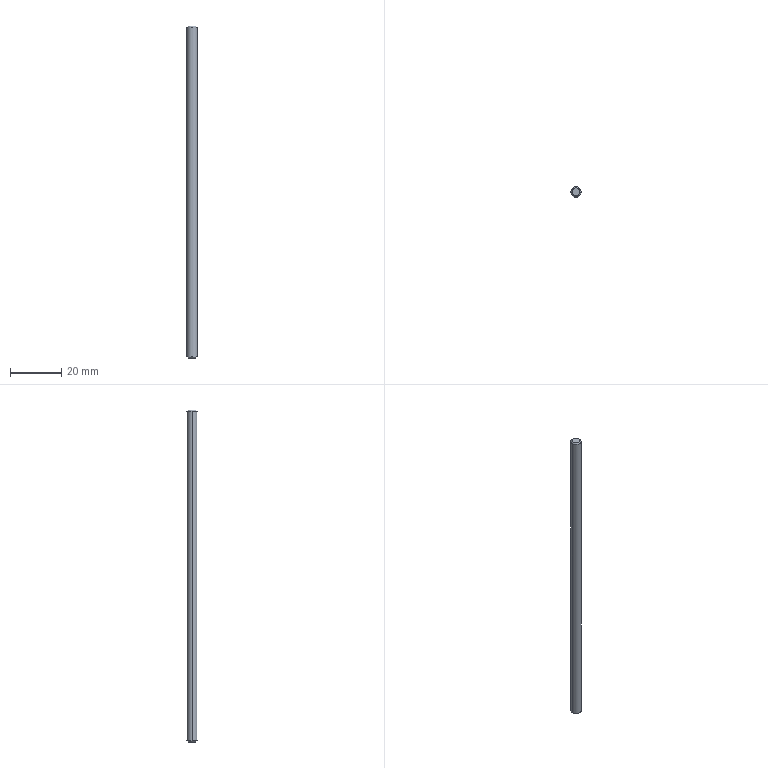Part | STEP file | 11-FG-B08311 | 1 solid | 8 faces | box 4 x 4 x 130 mm | volume 1631 mm3 | cone 4 | cylinder 2 | plane 2 | commonest cylinder face diameters 4 x2
STEP:
#1=CARTESIAN_POINT('',(-1.5,0.,0.));
#2=VERTEX_POINT('',#1);
#3=CARTESIAN_POINT('',(1.5,0.,0.));
#4=VERTEX_POINT('',#3);
#5=CARTESIAN_POINT('',(0.,0.,0.));
#6=DIRECTION('',(0.,0.,-1.));
#7=DIRECTION('',(1.,0.,0.));
#8=AXIS2_PLACEMENT_3D('',#5,#6,#7);
#9=CIRCLE('',#8,1.5);
#10=EDGE_CURVE('',#2,#4,#9,.T.);
#11=ORIENTED_EDGE('',*,*,#10,.F.);
#12=CARTESIAN_POINT('',(-2.,0.,0.5));
#13=VERTEX_POINT('',#12);
#14=CARTESIAN_POINT('',(-2.,0.,0.5));
#15=DIRECTION('',(-0.7071,0.,0.7071));
#16=VECTOR('',#15,1000.);
#17=LINE('',#14,#16);
#18=EDGE_CURVE('',#2,#13,#17,.T.);
#19=ORIENTED_EDGE('',*,*,#18,.T.);
#20=CARTESIAN_POINT('',(2.,0.,0.5));
#21=VERTEX_POINT('',#20);
#22=CARTESIAN_POINT('',(0.,0.,0.5));
#23=DIRECTION('',(0.,0.,1.));
#24=DIRECTION('',(1.,0.,0.));
#25=AXIS2_PLACEMENT_3D('',#22,#23,#24);
#26=CIRCLE('',#25,2.);
#27=EDGE_CURVE('',#21,#13,#26,.T.);
#28=ORIENTED_EDGE('',*,*,#27,.F.);
#29=CARTESIAN_POINT('',(2.,0.,0.5));
#30=DIRECTION('',(0.7071,0.,0.7071));
#31=VECTOR('',#30,1000.);
#32=LINE('',#29,#31);
#33=EDGE_CURVE('',#4,#21,#32,.T.);
#34=ORIENTED_EDGE('',*,*,#33,.F.);
#35=EDGE_LOOP('',(#11,#19,#28,#34));
#36=FACE_OUTER_BOUND('',#35,.T.);
#37=CARTESIAN_POINT('',(0.,0.,0.5));
#38=DIRECTION('',(0.,0.,1.));
#39=DIRECTION('',(1.,0.,0.));
#40=AXIS2_PLACEMENT_3D('',#37,#38,#39);
#41=CONICAL_SURFACE('',#40,2.,0.7854);
#42=ADVANCED_FACE('',(#36),#41,.T.);
#43=CARTESIAN_POINT('',(1.5,0.,130.));
#44=VERTEX_POINT('',#43);
#45=CARTESIAN_POINT('',(-1.5,0.,130.));
#46=VERTEX_POINT('',#45);
#47=CARTESIAN_POINT('',(0.,0.,130.));
#48=DIRECTION('',(0.,0.,1.));
#49=DIRECTION('',(1.,0.,0.));
#50=AXIS2_PLACEMENT_3D('',#47,#48,#49);
#51=CIRCLE('',#50,1.5);
#52=EDGE_CURVE('',#44,#46,#51,.T.);
#53=ORIENTED_EDGE('',*,*,#52,.F.);
#54=CARTESIAN_POINT('',(2.,0.,129.5));
#55=VERTEX_POINT('',#54);
#56=CARTESIAN_POINT('',(1.5,0.,130.));
#57=DIRECTION('',(0.7071,0.,-0.7071));
#58=VECTOR('',#57,1000.);
#59=LINE('',#56,#58);
#60=EDGE_CURVE('',#44,#55,#59,.T.);
#61=ORIENTED_EDGE('',*,*,#60,.T.);
#62=CARTESIAN_POINT('',(-2.,0.,129.5));
#63=VERTEX_POINT('',#62);
#64=CARTESIAN_POINT('',(0.,0.,129.5));
#65=DIRECTION('',(0.,0.,-1.));
#66=DIRECTION('',(1.,0.,0.));
#67=AXIS2_PLACEMENT_3D('',#64,#65,#66);
#68=CIRCLE('',#67,2.);
#69=EDGE_CURVE('',#63,#55,#68,.T.);
#70=ORIENTED_EDGE('',*,*,#69,.F.);
#71=CARTESIAN_POINT('',(-1.5,0.,130.));
#72=DIRECTION('',(-0.7071,0.,-0.7071));
#73=VECTOR('',#72,1000.);
#74=LINE('',#71,#73);
#75=EDGE_CURVE('',#46,#63,#74,.T.);
#76=ORIENTED_EDGE('',*,*,#75,.F.);
#77=EDGE_LOOP('',(#53,#61,#70,#76));
#78=FACE_OUTER_BOUND('',#77,.T.);
#79=CARTESIAN_POINT('',(0.,0.,130.));
#80=DIRECTION('',(0.,0.,-1.));
#81=DIRECTION('',(-1.,0.,0.));
#82=AXIS2_PLACEMENT_3D('',#79,#80,#81);
#83=CONICAL_SURFACE('',#82,1.5,0.7854);
#84=ADVANCED_FACE('',(#78),#83,.T.);
#85=ORIENTED_EDGE('',*,*,#69,.T.);
#86=CARTESIAN_POINT('',(2.,0.,130.));
#87=DIRECTION('',(0.,0.,-1.));
#88=VECTOR('',#87,1000.);
#89=LINE('',#86,#88);
#90=EDGE_CURVE('',#55,#21,#89,.T.);
#91=ORIENTED_EDGE('',*,*,#90,.T.);
#92=ORIENTED_EDGE('',*,*,#27,.T.);
#93=CARTESIAN_POINT('',(-2.,0.,130.));
#94=DIRECTION('',(0.,0.,-1.));
#95=VECTOR('',#94,1000.);
#96=LINE('',#93,#95);
#97=EDGE_CURVE('',#63,#13,#96,.T.);
#98=ORIENTED_EDGE('',*,*,#97,.F.);
#99=EDGE_LOOP('',(#85,#91,#92,#98));
#100=FACE_OUTER_BOUND('',#99,.T.);
#101=CARTESIAN_POINT('',(0.,0.,130.));
#102=DIRECTION('',(0.,0.,-1.));
#103=DIRECTION('',(-1.,0.,0.));
#104=AXIS2_PLACEMENT_3D('',#101,#102,#103);
#105=CYLINDRICAL_SURFACE('',#104,2.);
#106=ADVANCED_FACE('',(#100),#105,.T.);
#107=ORIENTED_EDGE('',*,*,#90,.F.);
#108=CARTESIAN_POINT('',(0.,0.,129.5));
#109=DIRECTION('',(0.,0.,-1.));
#110=DIRECTION('',(1.,0.,0.));
#111=AXIS2_PLACEMENT_3D('',#108,#109,#110);
#112=CIRCLE('',#111,2.);
#113=EDGE_CURVE('',#55,#63,#112,.T.);
#114=ORIENTED_EDGE('',*,*,#113,.T.);
#115=ORIENTED_EDGE('',*,*,#97,.T.);
#116=CARTESIAN_POINT('',(0.,0.,0.5));
#117=DIRECTION('',(0.,0.,1.));
#118=DIRECTION('',(1.,0.,0.));
#119=AXIS2_PLACEMENT_3D('',#116,#117,#118);
#120=CIRCLE('',#119,2.);
#121=EDGE_CURVE('',#13,#21,#120,.T.);
#122=ORIENTED_EDGE('',*,*,#121,.T.);
#123=EDGE_LOOP('',(#107,#114,#115,#122));
#124=FACE_OUTER_BOUND('',#123,.T.);
#125=CARTESIAN_POINT('',(0.,0.,130.));
#126=DIRECTION('',(0.,0.,-1.));
#127=DIRECTION('',(-1.,0.,0.));
#128=AXIS2_PLACEMENT_3D('',#125,#126,#127);
#129=CYLINDRICAL_SURFACE('',#128,2.);
#130=ADVANCED_FACE('',(#124),#129,.T.);
#131=CARTESIAN_POINT('',(0.,0.,130.));
#132=DIRECTION('',(0.,0.,1.));
#133=DIRECTION('',(1.,0.,0.));
#134=AXIS2_PLACEMENT_3D('',#131,#132,#133);
#135=CIRCLE('',#134,1.5);
#136=EDGE_CURVE('',#46,#44,#135,.T.);
#137=ORIENTED_EDGE('',*,*,#136,.T.);
#138=ORIENTED_EDGE('',*,*,#52,.T.);
#139=EDGE_LOOP('',(#137,#138));
#140=FACE_OUTER_BOUND('',#139,.T.);
#141=CARTESIAN_POINT('',(0.,0.,130.));
#142=DIRECTION('',(0.,0.,1.));
#143=DIRECTION('',(1.,0.,0.));
#144=AXIS2_PLACEMENT_3D('',#141,#142,#143);
#145=PLANE('',#144);
#146=ADVANCED_FACE('',(#140),#145,.T.);
#147=CARTESIAN_POINT('',(0.,0.,0.));
#148=DIRECTION('',(0.,0.,-1.));
#149=DIRECTION('',(1.,0.,0.));
#150=AXIS2_PLACEMENT_3D('',#147,#148,#149);
#151=CIRCLE('',#150,1.5);
#152=EDGE_CURVE('',#4,#2,#151,.T.);
#153=ORIENTED_EDGE('',*,*,#152,.T.);
#154=ORIENTED_EDGE('',*,*,#10,.T.);
#155=EDGE_LOOP('',(#153,#154));
#156=FACE_OUTER_BOUND('',#155,.T.);
#157=CARTESIAN_POINT('',(0.,0.,0.));
#158=DIRECTION('',(0.,0.,1.));
#159=DIRECTION('',(1.,0.,0.));
#160=AXIS2_PLACEMENT_3D('',#157,#158,#159);
#161=PLANE('',#160);
#162=ADVANCED_FACE('',(#156),#161,.F.);
#163=ORIENTED_EDGE('',*,*,#60,.F.);
#164=ORIENTED_EDGE('',*,*,#136,.F.);
#165=ORIENTED_EDGE('',*,*,#75,.T.);
#166=ORIENTED_EDGE('',*,*,#113,.F.);
#167=EDGE_LOOP('',(#163,#164,#165,#166));
#168=FACE_OUTER_BOUND('',#167,.T.);
#169=CARTESIAN_POINT('',(0.,0.,130.));
#170=DIRECTION('',(0.,0.,-1.));
#171=DIRECTION('',(-1.,0.,0.));
#172=AXIS2_PLACEMENT_3D('',#169,#170,#171);
#173=CONICAL_SURFACE('',#172,1.5,0.7854);
#174=ADVANCED_FACE('',(#168),#173,.T.);
#175=ORIENTED_EDGE('',*,*,#18,.F.);
#176=ORIENTED_EDGE('',*,*,#152,.F.);
#177=ORIENTED_EDGE('',*,*,#33,.T.);
#178=ORIENTED_EDGE('',*,*,#121,.F.);
#179=EDGE_LOOP('',(#175,#176,#177,#178));
#180=FACE_OUTER_BOUND('',#179,.T.);
#181=CARTESIAN_POINT('',(0.,0.,0.5));
#182=DIRECTION('',(0.,0.,1.));
#183=DIRECTION('',(1.,0.,0.));
#184=AXIS2_PLACEMENT_3D('',#181,#182,#183);
#185=CONICAL_SURFACE('',#184,2.,0.7854);
#186=ADVANCED_FACE('',(#180),#185,.T.);
#187=CLOSED_SHELL('',(#42,#84,#106,#130,#146,#162,#174,#186));
#188=MANIFOLD_SOLID_BREP('',#187);
#189=CARTESIAN_POINT('',(0.,0.,0.));
#190=DIRECTION('',(0.,0.,1.));
#191=DIRECTION('',(1.,0.,0.));
#192=AXIS2_PLACEMENT_3D('',#189,#190,#191);
#193=(LENGTH_UNIT()NAMED_UNIT(*)SI_UNIT(.MILLI.,.METRE.));
#194=UNCERTAINTY_MEASURE_WITH_UNIT(LENGTH_MEASURE(0.00001),#193,'','');
#195=(NAMED_UNIT(*)PLANE_ANGLE_UNIT()SI_UNIT($,.RADIAN.));
#196=(NAMED_UNIT(*)SI_UNIT($,.STERADIAN.)SOLID_ANGLE_UNIT());
#197=(GEOMETRIC_REPRESENTATION_CONTEXT(3)GLOBAL_UNCERTAINTY_ASSIGNED_CONTEXT((#194))GLOBAL_UNIT_ASSIGNED_CONTEXT((#193,#195,#196))REPRESENTATION_CONTEXT('',''));
#198=ADVANCED_BREP_SHAPE_REPRESENTATION('',(#188,#192),#197);